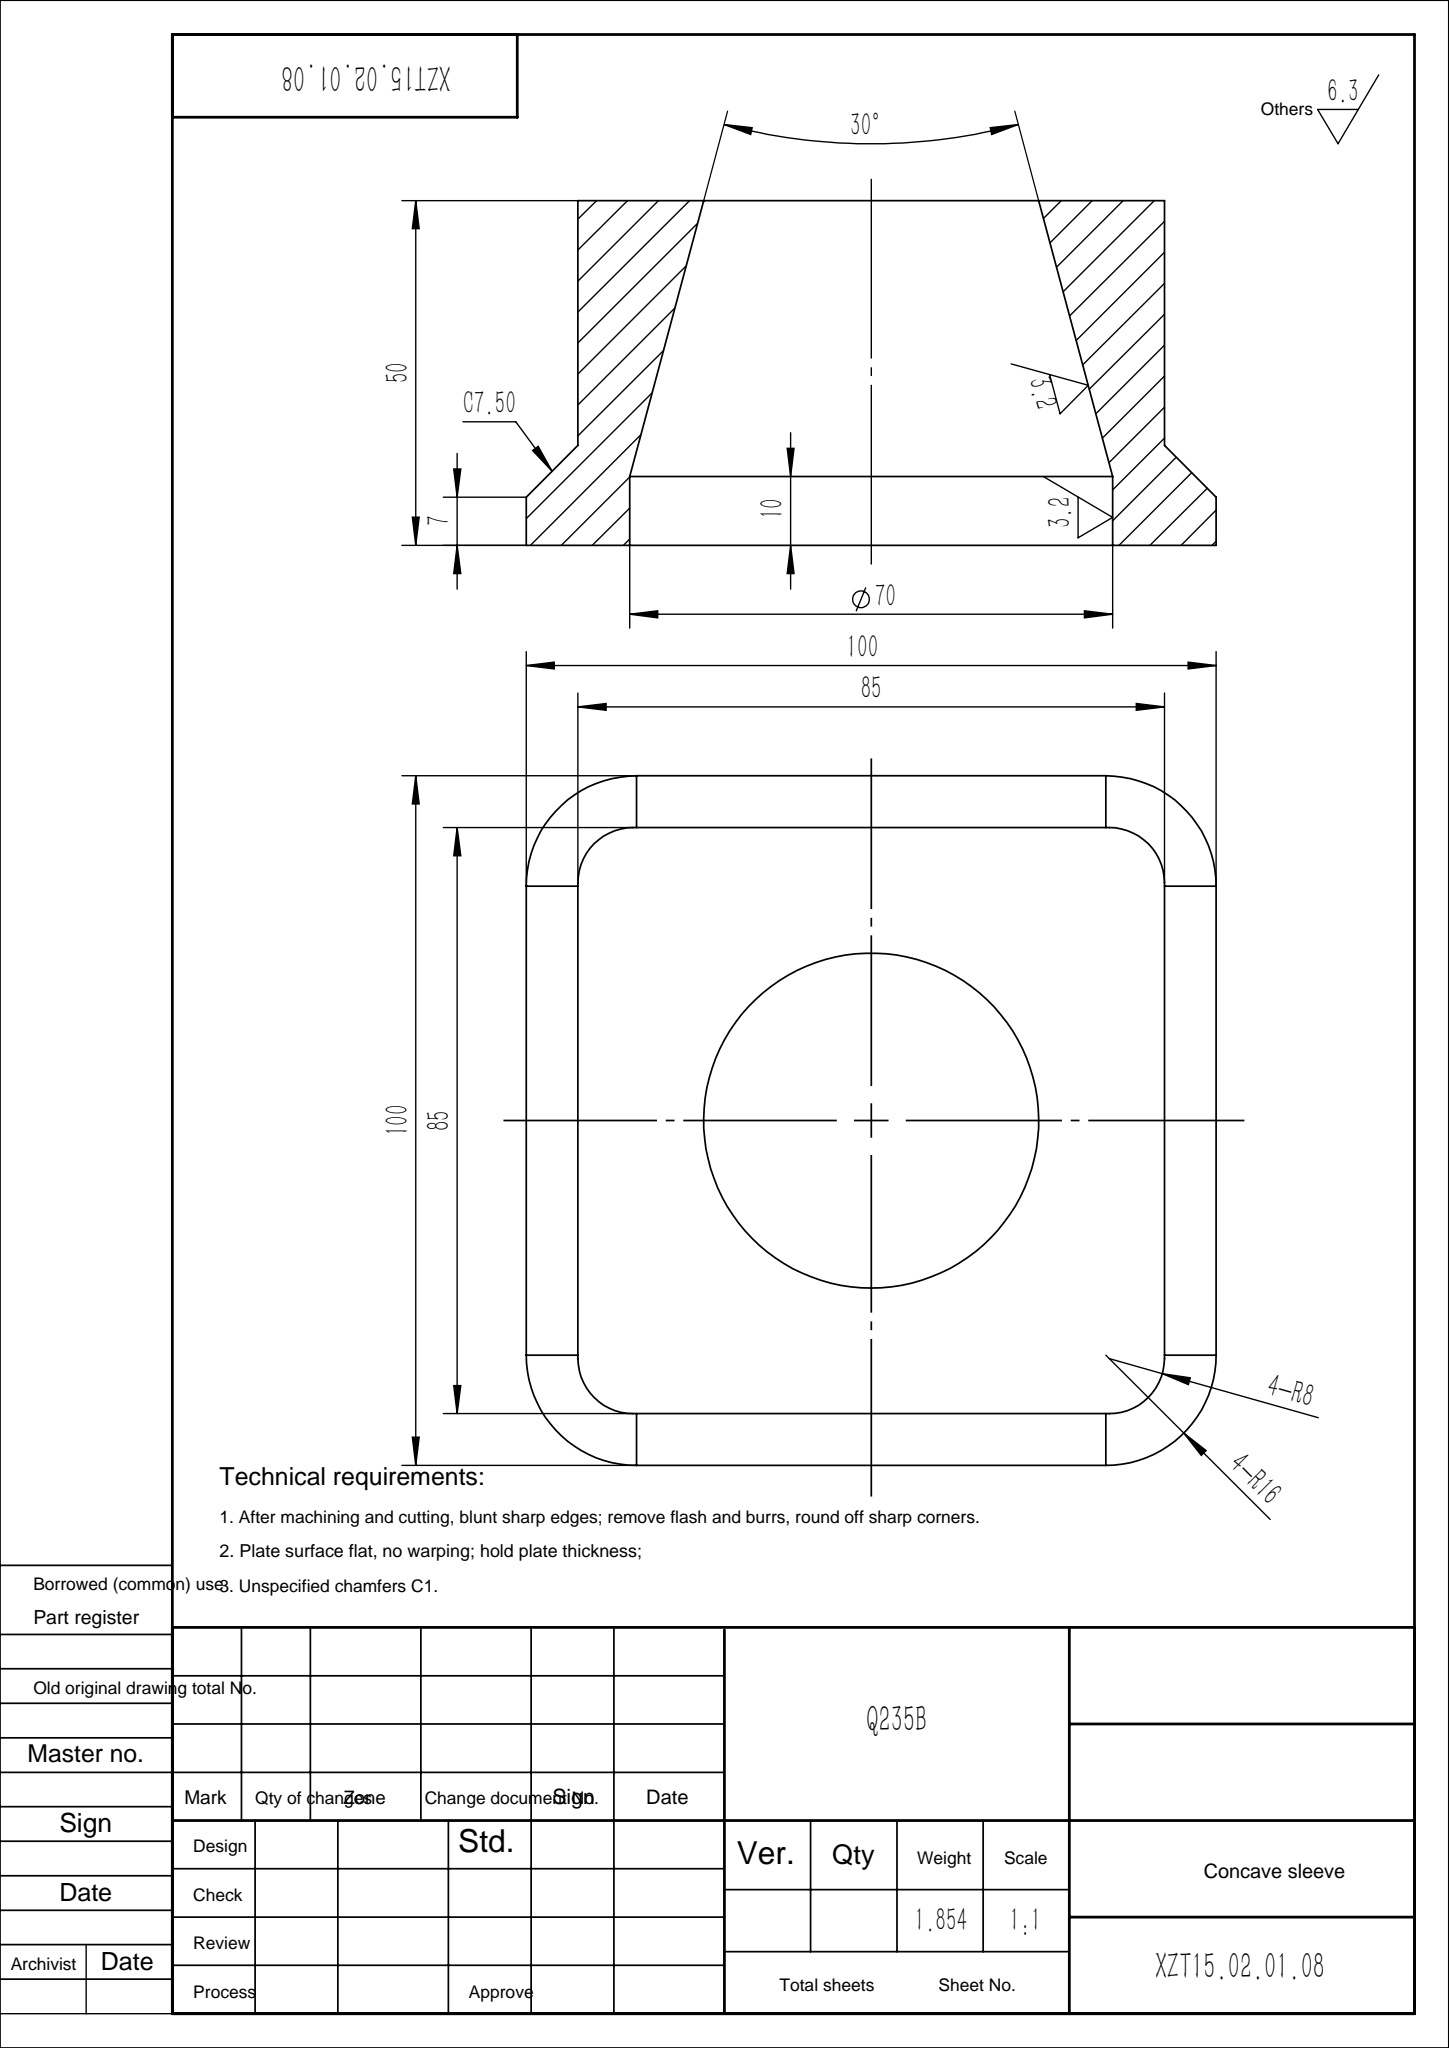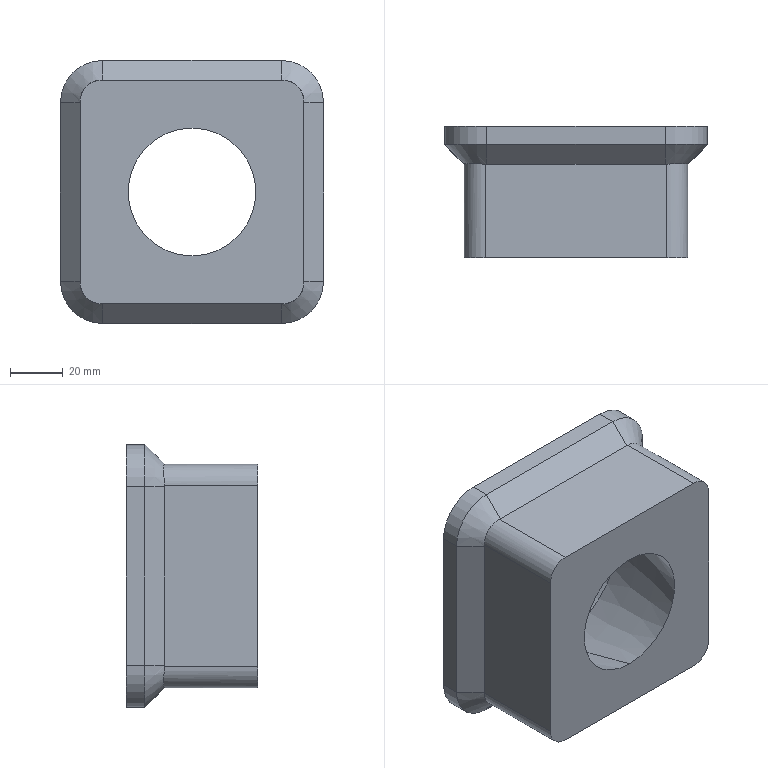Part | SolidWorks | features Chamfer 1, Extrusion 1, ICE 1, RevCut 1 | 1 solid | 30 faces | box 100 x 50 x 100 mm | volume 236221 mm3 | plane 14 | cylinder 10 | cone 6 | commonest cylinder face diameters 16 x4 32 x4 70 x2
STEP:
#1=CARTESIAN_POINT('',(0.,-50.,24.282));
#2=VERTEX_POINT('',#1);
#3=CARTESIAN_POINT('',(0.,-50.,-24.282));
#4=VERTEX_POINT('',#3);
#5=CARTESIAN_POINT('',(0.,-50.,0.));
#6=DIRECTION('',(0.,-1.,0.));
#7=DIRECTION('',(0.,0.,-1.));
#8=AXIS2_PLACEMENT_3D('',#5,#6,#7);
#9=CIRCLE('',#8,24.282);
#10=EDGE_CURVE('',#2,#4,#9,.T.);
#11=ORIENTED_EDGE('',*,*,#10,.T.);
#12=CARTESIAN_POINT('',(0.,-10.,-35.));
#13=VERTEX_POINT('',#12);
#14=CARTESIAN_POINT('',(0.,-10.,-35.));
#15=DIRECTION('',(0.,0.9659,-0.2588));
#16=VECTOR('',#15,1000.);
#17=LINE('',#14,#16);
#18=EDGE_CURVE('',#4,#13,#17,.T.);
#19=ORIENTED_EDGE('',*,*,#18,.T.);
#20=CARTESIAN_POINT('',(0.,-10.,35.));
#21=VERTEX_POINT('',#20);
#22=CARTESIAN_POINT('',(0.,-10.,0.));
#23=DIRECTION('',(0.,-1.,0.));
#24=DIRECTION('',(0.,0.,-1.));
#25=AXIS2_PLACEMENT_3D('',#22,#23,#24);
#26=CIRCLE('',#25,35.);
#27=EDGE_CURVE('',#21,#13,#26,.T.);
#28=ORIENTED_EDGE('',*,*,#27,.F.);
#29=CARTESIAN_POINT('',(0.,-10.,35.));
#30=DIRECTION('',(0.,0.9659,0.2588));
#31=VECTOR('',#30,1000.);
#32=LINE('',#29,#31);
#33=EDGE_CURVE('',#2,#21,#32,.T.);
#34=ORIENTED_EDGE('',*,*,#33,.F.);
#35=EDGE_LOOP('',(#11,#19,#28,#34));
#36=FACE_OUTER_BOUND('',#35,.T.);
#37=CARTESIAN_POINT('',(0.,-10.,0.));
#38=DIRECTION('',(0.,1.,0.));
#39=DIRECTION('',(0.,0.,1.));
#40=AXIS2_PLACEMENT_3D('',#37,#38,#39);
#41=CONICAL_SURFACE('',#40,35.,0.2618);
#42=ADVANCED_FACE('',(#36),#41,.F.);
#43=CARTESIAN_POINT('',(0.,0.,35.));
#44=VERTEX_POINT('',#43);
#45=CARTESIAN_POINT('',(0.,0.,-35.));
#46=VERTEX_POINT('',#45);
#47=CARTESIAN_POINT('',(0.,0.,0.));
#48=DIRECTION('',(0.,-1.,0.));
#49=DIRECTION('',(0.,0.,-1.));
#50=AXIS2_PLACEMENT_3D('',#47,#48,#49);
#51=CIRCLE('',#50,35.);
#52=EDGE_CURVE('',#44,#46,#51,.T.);
#53=ORIENTED_EDGE('',*,*,#52,.F.);
#54=CARTESIAN_POINT('',(0.,-50.,35.));
#55=DIRECTION('',(0.,-1.,0.));
#56=VECTOR('',#55,1000.);
#57=LINE('',#54,#56);
#58=EDGE_CURVE('',#44,#21,#57,.T.);
#59=ORIENTED_EDGE('',*,*,#58,.T.);
#60=ORIENTED_EDGE('',*,*,#27,.T.);
#61=CARTESIAN_POINT('',(0.,-50.,-35.));
#62=DIRECTION('',(0.,-1.,0.));
#63=VECTOR('',#62,1000.);
#64=LINE('',#61,#63);
#65=EDGE_CURVE('',#46,#13,#64,.T.);
#66=ORIENTED_EDGE('',*,*,#65,.F.);
#67=EDGE_LOOP('',(#53,#59,#60,#66));
#68=FACE_OUTER_BOUND('',#67,.T.);
#69=CARTESIAN_POINT('',(0.,-50.,0.));
#70=DIRECTION('',(0.,-1.,0.));
#71=DIRECTION('',(0.,0.,-1.));
#72=AXIS2_PLACEMENT_3D('',#69,#70,#71);
#73=CYLINDRICAL_SURFACE('',#72,35.);
#74=ADVANCED_FACE('',(#68),#73,.F.);
#75=CARTESIAN_POINT('',(-50.,-7.,34.));
#76=VERTEX_POINT('',#75);
#77=CARTESIAN_POINT('',(-50.,0.,34.));
#78=VERTEX_POINT('',#77);
#79=CARTESIAN_POINT('',(-50.,-15.,34.));
#80=DIRECTION('',(0.,1.,0.));
#81=VECTOR('',#80,1000.);
#82=LINE('',#79,#81);
#83=EDGE_CURVE('',#76,#78,#82,.T.);
#84=ORIENTED_EDGE('',*,*,#83,.F.);
#85=CARTESIAN_POINT('',(-34.,-7.,50.));
#86=VERTEX_POINT('',#85);
#87=CARTESIAN_POINT('',(-34.,-7.,34.));
#88=DIRECTION('',(0.,1.,0.));
#89=DIRECTION('',(0.,0.,-1.));
#90=AXIS2_PLACEMENT_3D('',#87,#88,#89);
#91=CIRCLE('',#90,16.);
#92=EDGE_CURVE('',#76,#86,#91,.T.);
#93=ORIENTED_EDGE('',*,*,#92,.T.);
#94=CARTESIAN_POINT('',(-34.,0.,50.));
#95=VERTEX_POINT('',#94);
#96=CARTESIAN_POINT('',(-34.,-15.,50.));
#97=DIRECTION('',(0.,1.,0.));
#98=VECTOR('',#97,1000.);
#99=LINE('',#96,#98);
#100=EDGE_CURVE('',#86,#95,#99,.T.);
#101=ORIENTED_EDGE('',*,*,#100,.T.);
#102=CARTESIAN_POINT('',(-34.,0.,34.));
#103=DIRECTION('',(0.,1.,0.));
#104=DIRECTION('',(0.,0.,-1.));
#105=AXIS2_PLACEMENT_3D('',#102,#103,#104);
#106=CIRCLE('',#105,16.);
#107=EDGE_CURVE('',#78,#95,#106,.T.);
#108=ORIENTED_EDGE('',*,*,#107,.F.);
#109=EDGE_LOOP('',(#84,#93,#101,#108));
#110=FACE_OUTER_BOUND('',#109,.T.);
#111=CARTESIAN_POINT('',(-34.,-15.,34.));
#112=DIRECTION('',(0.,1.,0.));
#113=DIRECTION('',(0.,0.,1.));
#114=AXIS2_PLACEMENT_3D('',#111,#112,#113);
#115=CYLINDRICAL_SURFACE('',#114,16.);
#116=ADVANCED_FACE('',(#110),#115,.T.);
#117=CARTESIAN_POINT('',(-50.,-7.,-34.));
#118=VERTEX_POINT('',#117);
#119=CARTESIAN_POINT('',(-50.,0.,-34.));
#120=VERTEX_POINT('',#119);
#121=CARTESIAN_POINT('',(-50.,-15.,-34.));
#122=DIRECTION('',(0.,1.,0.));
#123=VECTOR('',#122,1000.);
#124=LINE('',#121,#123);
#125=EDGE_CURVE('',#118,#120,#124,.T.);
#126=ORIENTED_EDGE('',*,*,#125,.F.);
#127=CARTESIAN_POINT('',(-50.,-7.,34.));
#128=DIRECTION('',(0.,0.,1.));
#129=VECTOR('',#128,1000.);
#130=LINE('',#127,#129);
#131=EDGE_CURVE('',#118,#76,#130,.T.);
#132=ORIENTED_EDGE('',*,*,#131,.T.);
#133=ORIENTED_EDGE('',*,*,#83,.T.);
#134=CARTESIAN_POINT('',(-50.,0.,34.));
#135=DIRECTION('',(0.,0.,1.));
#136=VECTOR('',#135,1000.);
#137=LINE('',#134,#136);
#138=EDGE_CURVE('',#120,#78,#137,.T.);
#139=ORIENTED_EDGE('',*,*,#138,.F.);
#140=EDGE_LOOP('',(#126,#132,#133,#139));
#141=FACE_OUTER_BOUND('',#140,.T.);
#142=CARTESIAN_POINT('',(-50.,-15.,34.));
#143=DIRECTION('',(-1.,0.,0.));
#144=DIRECTION('',(0.,0.,1.));
#145=AXIS2_PLACEMENT_3D('',#142,#143,#144);
#146=PLANE('',#145);
#147=ADVANCED_FACE('',(#141),#146,.T.);
#148=CARTESIAN_POINT('',(-34.,-7.,-50.));
#149=VERTEX_POINT('',#148);
#150=CARTESIAN_POINT('',(-34.,0.,-50.));
#151=VERTEX_POINT('',#150);
#152=CARTESIAN_POINT('',(-34.,-15.,-50.));
#153=DIRECTION('',(0.,1.,0.));
#154=VECTOR('',#153,1000.);
#155=LINE('',#152,#154);
#156=EDGE_CURVE('',#149,#151,#155,.T.);
#157=ORIENTED_EDGE('',*,*,#156,.F.);
#158=CARTESIAN_POINT('',(-34.,-7.,-34.));
#159=DIRECTION('',(0.,1.,0.));
#160=DIRECTION('',(0.,0.,-1.));
#161=AXIS2_PLACEMENT_3D('',#158,#159,#160);
#162=CIRCLE('',#161,16.);
#163=EDGE_CURVE('',#149,#118,#162,.T.);
#164=ORIENTED_EDGE('',*,*,#163,.T.);
#165=ORIENTED_EDGE('',*,*,#125,.T.);
#166=CARTESIAN_POINT('',(-34.,0.,-34.));
#167=DIRECTION('',(0.,1.,0.));
#168=DIRECTION('',(0.,0.,1.));
#169=AXIS2_PLACEMENT_3D('',#166,#167,#168);
#170=CIRCLE('',#169,16.);
#171=EDGE_CURVE('',#151,#120,#170,.T.);
#172=ORIENTED_EDGE('',*,*,#171,.F.);
#173=EDGE_LOOP('',(#157,#164,#165,#172));
#174=FACE_OUTER_BOUND('',#173,.T.);
#175=CARTESIAN_POINT('',(-34.,-15.,-34.));
#176=DIRECTION('',(0.,1.,0.));
#177=DIRECTION('',(0.,0.,1.));
#178=AXIS2_PLACEMENT_3D('',#175,#176,#177);
#179=CYLINDRICAL_SURFACE('',#178,16.);
#180=ADVANCED_FACE('',(#174),#179,.T.);
#181=CARTESIAN_POINT('',(34.,-7.,-50.));
#182=VERTEX_POINT('',#181);
#183=CARTESIAN_POINT('',(34.,0.,-50.));
#184=VERTEX_POINT('',#183);
#185=CARTESIAN_POINT('',(34.,-15.,-50.));
#186=DIRECTION('',(0.,1.,0.));
#187=VECTOR('',#186,1000.);
#188=LINE('',#185,#187);
#189=EDGE_CURVE('',#182,#184,#188,.T.);
#190=ORIENTED_EDGE('',*,*,#189,.F.);
#191=CARTESIAN_POINT('',(34.,-7.,-50.));
#192=DIRECTION('',(-1.,0.,0.));
#193=VECTOR('',#192,1000.);
#194=LINE('',#191,#193);
#195=EDGE_CURVE('',#182,#149,#194,.T.);
#196=ORIENTED_EDGE('',*,*,#195,.T.);
#197=ORIENTED_EDGE('',*,*,#156,.T.);
#198=CARTESIAN_POINT('',(34.,0.,-50.));
#199=DIRECTION('',(-1.,0.,0.));
#200=VECTOR('',#199,1000.);
#201=LINE('',#198,#200);
#202=EDGE_CURVE('',#184,#151,#201,.T.);
#203=ORIENTED_EDGE('',*,*,#202,.F.);
#204=EDGE_LOOP('',(#190,#196,#197,#203));
#205=FACE_OUTER_BOUND('',#204,.T.);
#206=CARTESIAN_POINT('',(34.,-15.,-50.));
#207=DIRECTION('',(0.,0.,-1.));
#208=DIRECTION('',(-1.,0.,0.));
#209=AXIS2_PLACEMENT_3D('',#206,#207,#208);
#210=PLANE('',#209);
#211=ADVANCED_FACE('',(#205),#210,.T.);
#212=CARTESIAN_POINT('',(50.,-7.,-34.));
#213=VERTEX_POINT('',#212);
#214=CARTESIAN_POINT('',(50.,0.,-34.));
#215=VERTEX_POINT('',#214);
#216=CARTESIAN_POINT('',(50.,-15.,-34.));
#217=DIRECTION('',(0.,1.,0.));
#218=VECTOR('',#217,1000.);
#219=LINE('',#216,#218);
#220=EDGE_CURVE('',#213,#215,#219,.T.);
#221=ORIENTED_EDGE('',*,*,#220,.F.);
#222=CARTESIAN_POINT('',(34.,-7.,-34.));
#223=DIRECTION('',(0.,1.,0.));
#224=DIRECTION('',(0.,0.,-1.));
#225=AXIS2_PLACEMENT_3D('',#222,#223,#224);
#226=CIRCLE('',#225,16.);
#227=EDGE_CURVE('',#213,#182,#226,.T.);
#228=ORIENTED_EDGE('',*,*,#227,.T.);
#229=ORIENTED_EDGE('',*,*,#189,.T.);
#230=CARTESIAN_POINT('',(34.,0.,-34.));
#231=DIRECTION('',(0.,1.,0.));
#232=DIRECTION('',(0.,0.,1.));
#233=AXIS2_PLACEMENT_3D('',#230,#231,#232);
#234=CIRCLE('',#233,16.);
#235=EDGE_CURVE('',#215,#184,#234,.T.);
#236=ORIENTED_EDGE('',*,*,#235,.F.);
#237=EDGE_LOOP('',(#221,#228,#229,#236));
#238=FACE_OUTER_BOUND('',#237,.T.);
#239=CARTESIAN_POINT('',(34.,-15.,-34.));
#240=DIRECTION('',(0.,1.,0.));
#241=DIRECTION('',(0.,0.,1.));
#242=AXIS2_PLACEMENT_3D('',#239,#240,#241);
#243=CYLINDRICAL_SURFACE('',#242,16.);
#244=ADVANCED_FACE('',(#238),#243,.T.);
#245=CARTESIAN_POINT('',(50.,-7.,34.));
#246=VERTEX_POINT('',#245);
#247=CARTESIAN_POINT('',(50.,0.,34.));
#248=VERTEX_POINT('',#247);
#249=CARTESIAN_POINT('',(50.,-15.,34.));
#250=DIRECTION('',(0.,1.,0.));
#251=VECTOR('',#250,1000.);
#252=LINE('',#249,#251);
#253=EDGE_CURVE('',#246,#248,#252,.T.);
#254=ORIENTED_EDGE('',*,*,#253,.F.);
#255=CARTESIAN_POINT('',(50.,-7.,34.));
#256=DIRECTION('',(0.,0.,-1.));
#257=VECTOR('',#256,1000.);
#258=LINE('',#255,#257);
#259=EDGE_CURVE('',#246,#213,#258,.T.);
#260=ORIENTED_EDGE('',*,*,#259,.T.);
#261=ORIENTED_EDGE('',*,*,#220,.T.);
#262=CARTESIAN_POINT('',(50.,0.,34.));
#263=DIRECTION('',(0.,0.,-1.));
#264=VECTOR('',#263,1000.);
#265=LINE('',#262,#264);
#266=EDGE_CURVE('',#248,#215,#265,.T.);
#267=ORIENTED_EDGE('',*,*,#266,.F.);
#268=EDGE_LOOP('',(#254,#260,#261,#267));
#269=FACE_OUTER_BOUND('',#268,.T.);
#270=CARTESIAN_POINT('',(50.,-15.,34.));
#271=DIRECTION('',(1.,0.,0.));
#272=DIRECTION('',(0.,0.,-1.));
#273=AXIS2_PLACEMENT_3D('',#270,#271,#272);
#274=PLANE('',#273);
#275=ADVANCED_FACE('',(#269),#274,.T.);
#276=CARTESIAN_POINT('',(34.,-7.,50.));
#277=VERTEX_POINT('',#276);
#278=CARTESIAN_POINT('',(34.,0.,50.));
#279=VERTEX_POINT('',#278);
#280=CARTESIAN_POINT('',(34.,-15.,50.));
#281=DIRECTION('',(0.,1.,0.));
#282=VECTOR('',#281,1000.);
#283=LINE('',#280,#282);
#284=EDGE_CURVE('',#277,#279,#283,.T.);
#285=ORIENTED_EDGE('',*,*,#284,.F.);
#286=CARTESIAN_POINT('',(34.,-7.,34.));
#287=DIRECTION('',(0.,1.,0.));
#288=DIRECTION('',(0.,0.,-1.));
#289=AXIS2_PLACEMENT_3D('',#286,#287,#288);
#290=CIRCLE('',#289,16.);
#291=EDGE_CURVE('',#277,#246,#290,.T.);
#292=ORIENTED_EDGE('',*,*,#291,.T.);
#293=ORIENTED_EDGE('',*,*,#253,.T.);
#294=CARTESIAN_POINT('',(34.,0.,34.));
#295=DIRECTION('',(0.,1.,0.));
#296=DIRECTION('',(0.,0.,1.));
#297=AXIS2_PLACEMENT_3D('',#294,#295,#296);
#298=CIRCLE('',#297,16.);
#299=EDGE_CURVE('',#279,#248,#298,.T.);
#300=ORIENTED_EDGE('',*,*,#299,.F.);
#301=EDGE_LOOP('',(#285,#292,#293,#300));
#302=FACE_OUTER_BOUND('',#301,.T.);
#303=CARTESIAN_POINT('',(34.,-15.,34.));
#304=DIRECTION('',(0.,1.,0.));
#305=DIRECTION('',(0.,0.,1.));
#306=AXIS2_PLACEMENT_3D('',#303,#304,#305);
#307=CYLINDRICAL_SURFACE('',#306,16.);
#308=ADVANCED_FACE('',(#302),#307,.T.);
#309=ORIENTED_EDGE('',*,*,#100,.F.);
#310=CARTESIAN_POINT('',(34.,-7.,50.));
#311=DIRECTION('',(1.,0.,0.));
#312=VECTOR('',#311,1000.);
#313=LINE('',#310,#312);
#314=EDGE_CURVE('',#86,#277,#313,.T.);
#315=ORIENTED_EDGE('',*,*,#314,.T.);
#316=ORIENTED_EDGE('',*,*,#284,.T.);
#317=CARTESIAN_POINT('',(34.,0.,50.));
#318=DIRECTION('',(1.,0.,0.));
#319=VECTOR('',#318,1000.);
#320=LINE('',#317,#319);
#321=EDGE_CURVE('',#95,#279,#320,.T.);
#322=ORIENTED_EDGE('',*,*,#321,.F.);
#323=EDGE_LOOP('',(#309,#315,#316,#322));
#324=FACE_OUTER_BOUND('',#323,.T.);
#325=CARTESIAN_POINT('',(34.,-15.,50.));
#326=DIRECTION('',(0.,0.,1.));
#327=DIRECTION('',(1.,0.,0.));
#328=AXIS2_PLACEMENT_3D('',#325,#326,#327);
#329=PLANE('',#328);
#330=ADVANCED_FACE('',(#324),#329,.T.);
#331=CARTESIAN_POINT('',(0.,0.,0.));
#332=DIRECTION('',(0.,-1.,0.));
#333=DIRECTION('',(0.,0.,-1.));
#334=AXIS2_PLACEMENT_3D('',#331,#332,#333);
#335=CIRCLE('',#334,35.);
#336=EDGE_CURVE('',#46,#44,#335,.T.);
#337=ORIENTED_EDGE('',*,*,#336,.T.);
#338=ORIENTED_EDGE('',*,*,#52,.T.);
#339=EDGE_LOOP('',(#337,#338));
#340=FACE_BOUND('',#339,.T.);
#341=ORIENTED_EDGE('',*,*,#107,.T.);
#342=ORIENTED_EDGE('',*,*,#321,.T.);
#343=ORIENTED_EDGE('',*,*,#299,.T.);
#344=ORIENTED_EDGE('',*,*,#266,.T.);
#345=ORIENTED_EDGE('',*,*,#235,.T.);
#346=ORIENTED_EDGE('',*,*,#202,.T.);
#347=ORIENTED_EDGE('',*,*,#171,.T.);
#348=ORIENTED_EDGE('',*,*,#138,.T.);
#349=EDGE_LOOP('',(#341,#342,#343,#344,#345,#346,#347,#348));
#350=FACE_OUTER_BOUND('',#349,.T.);
#351=CARTESIAN_POINT('',(-34.,0.,34.));
#352=DIRECTION('',(0.,-1.,0.));
#353=DIRECTION('',(0.,0.,-1.));
#354=AXIS2_PLACEMENT_3D('',#351,#352,#353);
#355=PLANE('',#354);
#356=ADVANCED_FACE('',(#340,#350),#355,.F.);
#357=CARTESIAN_POINT('',(-42.5,-50.,-34.5));
#358=VERTEX_POINT('',#357);
#359=CARTESIAN_POINT('',(-42.5,-14.485,-34.5));
#360=VERTEX_POINT('',#359);
#361=CARTESIAN_POINT('',(-42.5,-50.,-34.5));
#362=DIRECTION('',(0.,1.,0.));
#363=VECTOR('',#362,1000.);
#364=LINE('',#361,#363);
#365=EDGE_CURVE('',#358,#360,#364,.T.);
#366=ORIENTED_EDGE('',*,*,#365,.T.);
#367=CARTESIAN_POINT('',(-34.5,-14.485,-42.5));
#368=VERTEX_POINT('',#367);
#369=CARTESIAN_POINT('',(-42.5,-14.485,-34.5));
#370=CARTESIAN_POINT('',(-42.5,-14.454,-35.028));
#371=CARTESIAN_POINT('',(-42.448,-14.427,-35.547));
#372=CARTESIAN_POINT('',(-42.296,-14.391,-36.314));
#373=CARTESIAN_POINT('',(-42.232,-14.38,-36.568));
#374=CARTESIAN_POINT('',(-42.08,-14.36,-37.072));
#375=CARTESIAN_POINT('',(-41.991,-14.351,-37.321));
#376=CARTESIAN_POINT('',(-41.691,-14.326,-38.045));
#377=CARTESIAN_POINT('',(-41.445,-14.314,-38.505));
#378=CARTESIAN_POINT('',(-41.009,-14.301,-39.158));
#379=CARTESIAN_POINT('',(-40.851,-14.298,-39.371));
#380=CARTESIAN_POINT('',(-40.518,-14.294,-39.778));
#381=CARTESIAN_POINT('',(-40.342,-14.293,-39.971));
#382=CARTESIAN_POINT('',(-39.79,-14.293,-40.524));
#383=CARTESIAN_POINT('',(-39.387,-14.297,-40.856));
#384=CARTESIAN_POINT('',(-38.51,-14.314,-41.443));
#385=CARTESIAN_POINT('',(-38.047,-14.326,-41.689));
#386=CARTESIAN_POINT('',(-37.326,-14.35,-41.989));
#387=CARTESIAN_POINT('',(-37.08,-14.36,-42.077));
#388=CARTESIAN_POINT('',(-36.579,-14.38,-42.23));
#389=CARTESIAN_POINT('',(-36.322,-14.391,-42.294));
#390=CARTESIAN_POINT('',(-35.549,-14.427,-42.448));
#391=CARTESIAN_POINT('',(-35.028,-14.454,-42.5));
#392=CARTESIAN_POINT('',(-34.5,-14.485,-42.5));
#393=B_SPLINE_CURVE_WITH_KNOTS('',3,(#369,#370,#371,#372,#373,#374,#375,#376,#377,#378,#379,#380,#381,#382,#383,#384,#385,#386,#387,#388,#389,#390,#391,#392),.UNSPECIFIED.,.F.,.F.,(4,2,2,2,2,2,2,2,2,2,2,4),(0.,0.001565,0.002348,0.003131,0.004696,0.005479,0.006262,0.007827,0.009393,0.01018,0.01096,0.01252),.UNSPECIFIED.);
#394=EDGE_CURVE('',#360,#368,#393,.T.);
#395=ORIENTED_EDGE('',*,*,#394,.T.);
#396=CARTESIAN_POINT('',(-34.5,-50.,-42.5));
#397=VERTEX_POINT('',#396);
#398=CARTESIAN_POINT('',(-34.5,-50.,-42.5));
#399=DIRECTION('',(0.,1.,0.));
#400=VECTOR('',#399,1000.);
#401=LINE('',#398,#400);
#402=EDGE_CURVE('',#397,#368,#401,.T.);
#403=ORIENTED_EDGE('',*,*,#402,.F.);
#404=CARTESIAN_POINT('',(-34.5,-50.,-34.5));
#405=DIRECTION('',(0.,-1.,0.));
#406=DIRECTION('',(0.,0.,1.));
#407=AXIS2_PLACEMENT_3D('',#404,#405,#406);
#408=CIRCLE('',#407,8.);
#409=EDGE_CURVE('',#358,#397,#408,.T.);
#410=ORIENTED_EDGE('',*,*,#409,.F.);
#411=EDGE_LOOP('',(#366,#395,#403,#410));
#412=FACE_OUTER_BOUND('',#411,.T.);
#413=CARTESIAN_POINT('',(-34.5,-50.,-34.5));
#414=DIRECTION('',(0.,1.,0.));
#415=DIRECTION('',(0.,0.,1.));
#416=AXIS2_PLACEMENT_3D('',#413,#414,#415);
#417=CYLINDRICAL_SURFACE('',#416,8.);
#418=ADVANCED_FACE('',(#412),#417,.T.);
#419=ORIENTED_EDGE('',*,*,#402,.T.);
#420=CARTESIAN_POINT('',(-34.,-14.5,-42.5));
#421=VERTEX_POINT('',#420);
#422=CARTESIAN_POINT('',(-34.5,-14.485,-42.5));
#423=CARTESIAN_POINT('',(-34.333,-14.495,-42.5));
#424=CARTESIAN_POINT('',(-34.166,-14.5,-42.5));
#425=CARTESIAN_POINT('',(-34.,-14.5,-42.5));
#426=B_SPLINE_CURVE_WITH_KNOTS('',3,(#422,#423,#424,#425),.UNSPECIFIED.,.F.,.F.,(4,4),(0.,0.0004968),.UNSPECIFIED.);
#427=EDGE_CURVE('',#368,#421,#426,.T.);
#428=ORIENTED_EDGE('',*,*,#427,.T.);
#429=CARTESIAN_POINT('',(34.,-14.5,-42.5));
#430=VERTEX_POINT('',#429);
#431=CARTESIAN_POINT('',(34.5,-14.5,-42.5));
#432=DIRECTION('',(1.,0.,0.));
#433=VECTOR('',#432,1000.);
#434=LINE('',#431,#433);
#435=EDGE_CURVE('',#421,#430,#434,.T.);
#436=ORIENTED_EDGE('',*,*,#435,.T.);
#437=CARTESIAN_POINT('',(34.5,-14.485,-42.5));
#438=VERTEX_POINT('',#437);
#439=CARTESIAN_POINT('',(34.,-14.5,-42.5));
#440=CARTESIAN_POINT('',(34.167,-14.5,-42.5));
#441=CARTESIAN_POINT('',(34.333,-14.495,-42.5));
#442=CARTESIAN_POINT('',(34.5,-14.485,-42.5));
#443=B_SPLINE_CURVE_WITH_KNOTS('',3,(#439,#440,#441,#442),.UNSPECIFIED.,.F.,.F.,(4,4),(0.,0.0005002),.UNSPECIFIED.);
#444=EDGE_CURVE('',#430,#438,#443,.T.);
#445=ORIENTED_EDGE('',*,*,#444,.T.);
#446=CARTESIAN_POINT('',(34.5,-50.,-42.5));
#447=VERTEX_POINT('',#446);
#448=CARTESIAN_POINT('',(34.5,-50.,-42.5));
#449=DIRECTION('',(0.,1.,0.));
#450=VECTOR('',#449,1000.);
#451=LINE('',#448,#450);
#452=EDGE_CURVE('',#447,#438,#451,.T.);
#453=ORIENTED_EDGE('',*,*,#452,.F.);
#454=CARTESIAN_POINT('',(34.5,-50.,-42.5));
#455=DIRECTION('',(1.,0.,0.));
#456=VECTOR('',#455,1000.);
#457=LINE('',#454,#456);
#458=EDGE_CURVE('',#397,#447,#457,.T.);
#459=ORIENTED_EDGE('',*,*,#458,.F.);
#460=EDGE_LOOP('',(#419,#428,#436,#445,#453,#459));
#461=FACE_OUTER_BOUND('',#460,.T.);
#462=CARTESIAN_POINT('',(34.5,-50.,-42.5));
#463=DIRECTION('',(0.,0.,1.));
#464=DIRECTION('',(1.,0.,0.));
#465=AXIS2_PLACEMENT_3D('',#462,#463,#464);
#466=PLANE('',#465);
#467=ADVANCED_FACE('',(#461),#466,.F.);
#468=ORIENTED_EDGE('',*,*,#452,.T.);
#469=CARTESIAN_POINT('',(42.5,-14.485,-34.5));
#470=VERTEX_POINT('',#469);
#471=CARTESIAN_POINT('',(34.5,-14.485,-42.5));
#472=CARTESIAN_POINT('',(35.027,-14.454,-42.5));
#473=CARTESIAN_POINT('',(35.546,-14.427,-42.448));
#474=CARTESIAN_POINT('',(36.313,-14.391,-42.296));
#475=CARTESIAN_POINT('',(36.567,-14.38,-42.233));
#476=CARTESIAN_POINT('',(37.07,-14.36,-42.08));
#477=CARTESIAN_POINT('',(37.319,-14.351,-41.992));
#478=CARTESIAN_POINT('',(38.043,-14.326,-41.692));
#479=CARTESIAN_POINT('',(38.502,-14.314,-41.447));
#480=CARTESIAN_POINT('',(39.155,-14.301,-41.011));
#481=CARTESIAN_POINT('',(39.368,-14.298,-40.854));
#482=CARTESIAN_POINT('',(39.775,-14.294,-40.52));
#483=CARTESIAN_POINT('',(39.971,-14.293,-40.343));
#484=CARTESIAN_POINT('',(40.531,-14.293,-39.783));
#485=CARTESIAN_POINT('',(40.861,-14.297,-39.379));
#486=CARTESIAN_POINT('',(41.296,-14.309,-38.729));
#487=CARTESIAN_POINT('',(41.43,-14.315,-38.505));
#488=CARTESIAN_POINT('',(41.678,-14.327,-38.041));
#489=CARTESIAN_POINT('',(41.791,-14.334,-37.802));
#490=CARTESIAN_POINT('',(42.091,-14.359,-37.077));
#491=CARTESIAN_POINT('',(42.243,-14.379,-36.58));
#492=CARTESIAN_POINT('',(42.447,-14.427,-35.555));
#493=CARTESIAN_POINT('',(42.5,-14.454,-35.027));
#494=CARTESIAN_POINT('',(42.5,-14.485,-34.5));
#495=B_SPLINE_CURVE_WITH_KNOTS('',3,(#471,#472,#473,#474,#475,#476,#477,#478,#479,#480,#481,#482,#483,#484,#485,#486,#487,#488,#489,#490,#491,#492,#493,#494),.UNSPECIFIED.,.F.,.F.,(4,2,2,2,2,2,2,2,2,2,2,4),(-0.006252,-0.004689,-0.003908,-0.003126,-0.001563,-0.000781,0.000000577,0.001564,0.002345,0.003127,0.00469,0.006254),.UNSPECIFIED.);
#496=EDGE_CURVE('',#438,#470,#495,.T.);
#497=ORIENTED_EDGE('',*,*,#496,.T.);
#498=CARTESIAN_POINT('',(42.5,-50.,-34.5));
#499=VERTEX_POINT('',#498);
#500=CARTESIAN_POINT('',(42.5,-50.,-34.5));
#501=DIRECTION('',(0.,1.,0.));
#502=VECTOR('',#501,1000.);
#503=LINE('',#500,#502);
#504=EDGE_CURVE('',#499,#470,#503,.T.);
#505=ORIENTED_EDGE('',*,*,#504,.F.);
#506=CARTESIAN_POINT('',(34.5,-50.,-34.5));
#507=DIRECTION('',(0.,-1.,0.));
#508=DIRECTION('',(0.,0.,-1.));
#509=AXIS2_PLACEMENT_3D('',#506,#507,#508);
#510=CIRCLE('',#509,8.);
#511=EDGE_CURVE('',#447,#499,#510,.T.);
#512=ORIENTED_EDGE('',*,*,#511,.F.);
#513=EDGE_LOOP('',(#468,#497,#505,#512));
#514=FACE_OUTER_BOUND('',#513,.T.);
#515=CARTESIAN_POINT('',(34.5,-50.,-34.5));
#516=DIRECTION('',(0.,1.,0.));
#517=DIRECTION('',(0.,0.,1.));
#518=AXIS2_PLACEMENT_3D('',#515,#516,#517);
#519=CYLINDRICAL_SURFACE('',#518,8.);
#520=ADVANCED_FACE('',(#514),#519,.T.);
#521=CARTESIAN_POINT('',(42.5,-14.5,-34.));
#522=VERTEX_POINT('',#521);
#523=CARTESIAN_POINT('',(42.5,-14.5,34.));
#524=VERTEX_POINT('',#523);
#525=CARTESIAN_POINT('',(42.5,-14.5,-34.5));
#526=DIRECTION('',(0.,0.,1.));
#527=VECTOR('',#526,1000.);
#528=LINE('',#525,#527);
#529=EDGE_CURVE('',#522,#524,#528,.T.);
#530=ORIENTED_EDGE('',*,*,#529,.T.);
#531=CARTESIAN_POINT('',(42.5,-14.485,34.5));
#532=VERTEX_POINT('',#531);
#533=CARTESIAN_POINT('',(42.5,-14.5,34.));
#534=CARTESIAN_POINT('',(42.5,-14.5,34.167));
#535=CARTESIAN_POINT('',(42.5,-14.495,34.333));
#536=CARTESIAN_POINT('',(42.5,-14.485,34.5));
#537=B_SPLINE_CURVE_WITH_KNOTS('',3,(#533,#534,#535,#536),.UNSPECIFIED.,.F.,.F.,(4,4),(0.,0.0005002),.UNSPECIFIED.);
#538=EDGE_CURVE('',#524,#532,#537,.T.);
#539=ORIENTED_EDGE('',*,*,#538,.T.);
#540=CARTESIAN_POINT('',(42.5,-50.,34.5));
#541=VERTEX_POINT('',#540);
#542=CARTESIAN_POINT('',(42.5,-50.,34.5));
#543=DIRECTION('',(0.,1.,0.));
#544=VECTOR('',#543,1000.);
#545=LINE('',#542,#544);
#546=EDGE_CURVE('',#541,#532,#545,.T.);
#547=ORIENTED_EDGE('',*,*,#546,.F.);
#548=CARTESIAN_POINT('',(42.5,-50.,-34.5));
#549=DIRECTION('',(0.,0.,1.));
#550=VECTOR('',#549,1000.);
#551=LINE('',#548,#550);
#552=EDGE_CURVE('',#499,#541,#551,.T.);
#553=ORIENTED_EDGE('',*,*,#552,.F.);
#554=ORIENTED_EDGE('',*,*,#504,.T.);
#555=CARTESIAN_POINT('',(42.5,-14.485,-34.5));
#556=CARTESIAN_POINT('',(42.5,-14.495,-34.333));
#557=CARTESIAN_POINT('',(42.5,-14.5,-34.166));
#558=CARTESIAN_POINT('',(42.5,-14.5,-34.));
#559=B_SPLINE_CURVE_WITH_KNOTS('',3,(#555,#556,#557,#558),.UNSPECIFIED.,.F.,.F.,(4,4),(0.,0.0004968),.UNSPECIFIED.);
#560=EDGE_CURVE('',#470,#522,#559,.T.);
#561=ORIENTED_EDGE('',*,*,#560,.T.);
#562=EDGE_LOOP('',(#530,#539,#547,#553,#554,#561));
#563=FACE_OUTER_BOUND('',#562,.T.);
#564=CARTESIAN_POINT('',(42.5,-50.,-34.5));
#565=DIRECTION('',(-1.,0.,0.));
#566=DIRECTION('',(0.,0.,1.));
#567=AXIS2_PLACEMENT_3D('',#564,#565,#566);
#568=PLANE('',#567);
#569=ADVANCED_FACE('',(#563),#568,.F.);
#570=ORIENTED_EDGE('',*,*,#546,.T.);
#571=CARTESIAN_POINT('',(34.5,-14.485,42.5));
#572=VERTEX_POINT('',#571);
#573=CARTESIAN_POINT('',(42.5,-14.485,34.5));
#574=CARTESIAN_POINT('',(42.5,-14.454,35.028));
#575=CARTESIAN_POINT('',(42.448,-14.427,35.547));
#576=CARTESIAN_POINT('',(42.296,-14.391,36.314));
#577=CARTESIAN_POINT('',(42.232,-14.38,36.568));
#578=CARTESIAN_POINT('',(42.08,-14.36,37.072));
#579=CARTESIAN_POINT('',(41.991,-14.351,37.321));
#580=CARTESIAN_POINT('',(41.691,-14.326,38.045));
#581=CARTESIAN_POINT('',(41.445,-14.314,38.505));
#582=CARTESIAN_POINT('',(41.009,-14.301,39.158));
#583=CARTESIAN_POINT('',(40.851,-14.298,39.371));
#584=CARTESIAN_POINT('',(40.518,-14.294,39.778));
#585=CARTESIAN_POINT('',(40.342,-14.293,39.971));
#586=CARTESIAN_POINT('',(39.79,-14.293,40.524));
#587=CARTESIAN_POINT('',(39.387,-14.297,40.856));
#588=CARTESIAN_POINT('',(38.51,-14.314,41.443));
#589=CARTESIAN_POINT('',(38.047,-14.326,41.689));
#590=CARTESIAN_POINT('',(37.326,-14.35,41.989));
#591=CARTESIAN_POINT('',(37.08,-14.36,42.077));
#592=CARTESIAN_POINT('',(36.579,-14.38,42.23));
#593=CARTESIAN_POINT('',(36.322,-14.391,42.294));
#594=CARTESIAN_POINT('',(35.549,-14.427,42.448));
#595=CARTESIAN_POINT('',(35.028,-14.454,42.5));
#596=CARTESIAN_POINT('',(34.5,-14.485,42.5));
#597=B_SPLINE_CURVE_WITH_KNOTS('',3,(#573,#574,#575,#576,#577,#578,#579,#580,#581,#582,#583,#584,#585,#586,#587,#588,#589,#590,#591,#592,#593,#594,#595,#596),.UNSPECIFIED.,.F.,.F.,(4,2,2,2,2,2,2,2,2,2,2,4),(0.,0.001565,0.002348,0.003131,0.004696,0.005479,0.006262,0.007827,0.009393,0.01018,0.01096,0.01252),.UNSPECIFIED.);
#598=EDGE_CURVE('',#532,#572,#597,.T.);
#599=ORIENTED_EDGE('',*,*,#598,.T.);
#600=CARTESIAN_POINT('',(34.5,-50.,42.5));
#601=VERTEX_POINT('',#600);
#602=CARTESIAN_POINT('',(34.5,-50.,42.5));
#603=DIRECTION('',(0.,1.,0.));
#604=VECTOR('',#603,1000.);
#605=LINE('',#602,#604);
#606=EDGE_CURVE('',#601,#572,#605,.T.);
#607=ORIENTED_EDGE('',*,*,#606,.F.);
#608=CARTESIAN_POINT('',(34.5,-50.,34.5));
#609=DIRECTION('',(0.,-1.,0.));
#610=DIRECTION('',(0.,0.,-1.));
#611=AXIS2_PLACEMENT_3D('',#608,#609,#610);
#612=CIRCLE('',#611,8.);
#613=EDGE_CURVE('',#541,#601,#612,.T.);
#614=ORIENTED_EDGE('',*,*,#613,.F.);
#615=EDGE_LOOP('',(#570,#599,#607,#614));
#616=FACE_OUTER_BOUND('',#615,.T.);
#617=CARTESIAN_POINT('',(34.5,-50.,34.5));
#618=DIRECTION('',(0.,1.,0.));
#619=DIRECTION('',(0.,0.,1.));
#620=AXIS2_PLACEMENT_3D('',#617,#618,#619);
#621=CYLINDRICAL_SURFACE('',#620,8.);
#622=ADVANCED_FACE('',(#616),#621,.T.);
#623=CARTESIAN_POINT('',(34.,-14.5,42.5));
#624=VERTEX_POINT('',#623);
#625=CARTESIAN_POINT('',(-34.,-14.5,42.5));
#626=VERTEX_POINT('',#625);
#627=CARTESIAN_POINT('',(34.5,-14.5,42.5));
#628=DIRECTION('',(-1.,0.,0.));
#629=VECTOR('',#628,1000.);
#630=LINE('',#627,#629);
#631=EDGE_CURVE('',#624,#626,#630,.T.);
#632=ORIENTED_EDGE('',*,*,#631,.T.);
#633=CARTESIAN_POINT('',(-34.5,-14.485,42.5));
#634=VERTEX_POINT('',#633);
#635=CARTESIAN_POINT('',(-34.,-14.5,42.5));
#636=CARTESIAN_POINT('',(-34.167,-14.5,42.5));
#637=CARTESIAN_POINT('',(-34.333,-14.495,42.5));
#638=CARTESIAN_POINT('',(-34.5,-14.485,42.5));
#639=B_SPLINE_CURVE_WITH_KNOTS('',3,(#635,#636,#637,#638),.UNSPECIFIED.,.F.,.F.,(4,4),(0.,0.0005002),.UNSPECIFIED.);
#640=EDGE_CURVE('',#626,#634,#639,.T.);
#641=ORIENTED_EDGE('',*,*,#640,.T.);
#642=CARTESIAN_POINT('',(-34.5,-50.,42.5));
#643=VERTEX_POINT('',#642);
#644=CARTESIAN_POINT('',(-34.5,-50.,42.5));
#645=DIRECTION('',(0.,1.,0.));
#646=VECTOR('',#645,1000.);
#647=LINE('',#644,#646);
#648=EDGE_CURVE('',#643,#634,#647,.T.);
#649=ORIENTED_EDGE('',*,*,#648,.F.);
#650=CARTESIAN_POINT('',(34.5,-50.,42.5));
#651=DIRECTION('',(-1.,0.,0.));
#652=VECTOR('',#651,1000.);
#653=LINE('',#650,#652);
#654=EDGE_CURVE('',#601,#643,#653,.T.);
#655=ORIENTED_EDGE('',*,*,#654,.F.);
#656=ORIENTED_EDGE('',*,*,#606,.T.);
#657=CARTESIAN_POINT('',(34.5,-14.485,42.5));
#658=CARTESIAN_POINT('',(34.333,-14.495,42.5));
#659=CARTESIAN_POINT('',(34.166,-14.5,42.5));
#660=CARTESIAN_POINT('',(34.,-14.5,42.5));
#661=B_SPLINE_CURVE_WITH_KNOTS('',3,(#657,#658,#659,#660),.UNSPECIFIED.,.F.,.F.,(4,4),(0.,0.0004968),.UNSPECIFIED.);
#662=EDGE_CURVE('',#572,#624,#661,.T.);
#663=ORIENTED_EDGE('',*,*,#662,.T.);
#664=EDGE_LOOP('',(#632,#641,#649,#655,#656,#663));
#665=FACE_OUTER_BOUND('',#664,.T.);
#666=CARTESIAN_POINT('',(34.5,-50.,42.5));
#667=DIRECTION('',(0.,0.,-1.));
#668=DIRECTION('',(-1.,0.,0.));
#669=AXIS2_PLACEMENT_3D('',#666,#667,#668);
#670=PLANE('',#669);
#671=ADVANCED_FACE('',(#665),#670,.F.);
#672=ORIENTED_EDGE('',*,*,#648,.T.);
#673=CARTESIAN_POINT('',(-42.5,-14.485,34.5));
#674=VERTEX_POINT('',#673);
#675=CARTESIAN_POINT('',(-34.5,-14.485,42.5));
#676=CARTESIAN_POINT('',(-35.028,-14.454,42.5));
#677=CARTESIAN_POINT('',(-35.547,-14.427,42.448));
#678=CARTESIAN_POINT('',(-36.314,-14.391,42.296));
#679=CARTESIAN_POINT('',(-36.568,-14.38,42.232));
#680=CARTESIAN_POINT('',(-37.072,-14.36,42.08));
#681=CARTESIAN_POINT('',(-37.321,-14.351,41.991));
#682=CARTESIAN_POINT('',(-38.045,-14.326,41.691));
#683=CARTESIAN_POINT('',(-38.505,-14.314,41.445));
#684=CARTESIAN_POINT('',(-39.158,-14.301,41.009));
#685=CARTESIAN_POINT('',(-39.371,-14.298,40.851));
#686=CARTESIAN_POINT('',(-39.778,-14.294,40.518));
#687=CARTESIAN_POINT('',(-39.971,-14.293,40.342));
#688=CARTESIAN_POINT('',(-40.524,-14.293,39.79));
#689=CARTESIAN_POINT('',(-40.856,-14.297,39.387));
#690=CARTESIAN_POINT('',(-41.443,-14.314,38.51));
#691=CARTESIAN_POINT('',(-41.689,-14.326,38.047));
#692=CARTESIAN_POINT('',(-41.989,-14.35,37.326));
#693=CARTESIAN_POINT('',(-42.077,-14.36,37.08));
#694=CARTESIAN_POINT('',(-42.23,-14.38,36.579));
#695=CARTESIAN_POINT('',(-42.294,-14.391,36.322));
#696=CARTESIAN_POINT('',(-42.448,-14.427,35.549));
#697=CARTESIAN_POINT('',(-42.5,-14.454,35.028));
#698=CARTESIAN_POINT('',(-42.5,-14.485,34.5));
#699=B_SPLINE_CURVE_WITH_KNOTS('',3,(#675,#676,#677,#678,#679,#680,#681,#682,#683,#684,#685,#686,#687,#688,#689,#690,#691,#692,#693,#694,#695,#696,#697,#698),.UNSPECIFIED.,.F.,.F.,(4,2,2,2,2,2,2,2,2,2,2,4),(0.,0.001565,0.002348,0.003131,0.004696,0.005479,0.006262,0.007827,0.009393,0.01018,0.01096,0.01252),.UNSPECIFIED.);
#700=EDGE_CURVE('',#634,#674,#699,.T.);
#701=ORIENTED_EDGE('',*,*,#700,.T.);
#702=CARTESIAN_POINT('',(-42.5,-50.,34.5));
#703=VERTEX_POINT('',#702);
#704=CARTESIAN_POINT('',(-42.5,-50.,34.5));
#705=DIRECTION('',(0.,1.,0.));
#706=VECTOR('',#705,1000.);
#707=LINE('',#704,#706);
#708=EDGE_CURVE('',#703,#674,#707,.T.);
#709=ORIENTED_EDGE('',*,*,#708,.F.);
#710=CARTESIAN_POINT('',(-34.5,-50.,34.5));
#711=DIRECTION('',(0.,-1.,0.));
#712=DIRECTION('',(0.,0.,-1.));
#713=AXIS2_PLACEMENT_3D('',#710,#711,#712);
#714=CIRCLE('',#713,8.);
#715=EDGE_CURVE('',#643,#703,#714,.T.);
#716=ORIENTED_EDGE('',*,*,#715,.F.);
#717=EDGE_LOOP('',(#672,#701,#709,#716));
#718=FACE_OUTER_BOUND('',#717,.T.);
#719=CARTESIAN_POINT('',(-34.5,-50.,34.5));
#720=DIRECTION('',(0.,1.,0.));
#721=DIRECTION('',(0.,0.,1.));
#722=AXIS2_PLACEMENT_3D('',#719,#720,#721);
#723=CYLINDRICAL_SURFACE('',#722,8.);
#724=ADVANCED_FACE('',(#718),#723,.T.);
#725=ORIENTED_EDGE('',*,*,#708,.T.);
#726=CARTESIAN_POINT('',(-42.5,-14.5,34.));
#727=VERTEX_POINT('',#726);
#728=CARTESIAN_POINT('',(-42.5,-14.485,34.5));
#729=CARTESIAN_POINT('',(-42.5,-14.495,34.333));
#730=CARTESIAN_POINT('',(-42.5,-14.5,34.166));
#731=CARTESIAN_POINT('',(-42.5,-14.5,34.));
#732=B_SPLINE_CURVE_WITH_KNOTS('',3,(#728,#729,#730,#731),.UNSPECIFIED.,.F.,.F.,(4,4),(0.,0.0004968),.UNSPECIFIED.);
#733=EDGE_CURVE('',#674,#727,#732,.T.);
#734=ORIENTED_EDGE('',*,*,#733,.T.);
#735=CARTESIAN_POINT('',(-42.5,-14.5,-34.));
#736=VERTEX_POINT('',#735);
#737=CARTESIAN_POINT('',(-42.5,-14.5,-34.5));
#738=DIRECTION('',(0.,0.,-1.));
#739=VECTOR('',#738,1000.);
#740=LINE('',#737,#739);
#741=EDGE_CURVE('',#727,#736,#740,.T.);
#742=ORIENTED_EDGE('',*,*,#741,.T.);
#743=CARTESIAN_POINT('',(-42.5,-14.5,-34.));
#744=CARTESIAN_POINT('',(-42.5,-14.5,-34.167));
#745=CARTESIAN_POINT('',(-42.5,-14.495,-34.333));
#746=CARTESIAN_POINT('',(-42.5,-14.485,-34.5));
#747=B_SPLINE_CURVE_WITH_KNOTS('',3,(#743,#744,#745,#746),.UNSPECIFIED.,.F.,.F.,(4,4),(0.,0.0005002),.UNSPECIFIED.);
#748=EDGE_CURVE('',#736,#360,#747,.T.);
#749=ORIENTED_EDGE('',*,*,#748,.T.);
#750=ORIENTED_EDGE('',*,*,#365,.F.);
#751=CARTESIAN_POINT('',(-42.5,-50.,-34.5));
#752=DIRECTION('',(0.,0.,-1.));
#753=VECTOR('',#752,1000.);
#754=LINE('',#751,#753);
#755=EDGE_CURVE('',#703,#358,#754,.T.);
#756=ORIENTED_EDGE('',*,*,#755,.F.);
#757=EDGE_LOOP('',(#725,#734,#742,#749,#750,#756));
#758=FACE_OUTER_BOUND('',#757,.T.);
#759=CARTESIAN_POINT('',(-42.5,-50.,-34.5));
#760=DIRECTION('',(1.,0.,0.));
#761=DIRECTION('',(0.,0.,-1.));
#762=AXIS2_PLACEMENT_3D('',#759,#760,#761);
#763=PLANE('',#762);
#764=ADVANCED_FACE('',(#758),#763,.F.);
#765=ORIENTED_EDGE('',*,*,#10,.F.);
#766=CARTESIAN_POINT('',(0.,-50.,0.));
#767=DIRECTION('',(0.,-1.,0.));
#768=DIRECTION('',(0.,0.,-1.));
#769=AXIS2_PLACEMENT_3D('',#766,#767,#768);
#770=CIRCLE('',#769,24.282);
#771=EDGE_CURVE('',#4,#2,#770,.T.);
#772=ORIENTED_EDGE('',*,*,#771,.F.);
#773=EDGE_LOOP('',(#765,#772));
#774=FACE_BOUND('',#773,.T.);
#775=ORIENTED_EDGE('',*,*,#409,.T.);
#776=ORIENTED_EDGE('',*,*,#458,.T.);
#777=ORIENTED_EDGE('',*,*,#511,.T.);
#778=ORIENTED_EDGE('',*,*,#552,.T.);
#779=ORIENTED_EDGE('',*,*,#613,.T.);
#780=ORIENTED_EDGE('',*,*,#654,.T.);
#781=ORIENTED_EDGE('',*,*,#715,.T.);
#782=ORIENTED_EDGE('',*,*,#755,.T.);
#783=EDGE_LOOP('',(#775,#776,#777,#778,#779,#780,#781,#782));
#784=FACE_OUTER_BOUND('',#783,.T.);
#785=CARTESIAN_POINT('',(-34.5,-50.,-34.5));
#786=DIRECTION('',(0.,1.,0.));
#787=DIRECTION('',(0.,0.,1.));
#788=AXIS2_PLACEMENT_3D('',#785,#786,#787);
#789=PLANE('',#788);
#790=ADVANCED_FACE('',(#774,#784),#789,.F.);
#791=ORIENTED_EDGE('',*,*,#58,.F.);
#792=ORIENTED_EDGE('',*,*,#336,.F.);
#793=ORIENTED_EDGE('',*,*,#65,.T.);
#794=CARTESIAN_POINT('',(0.,-10.,0.));
#795=DIRECTION('',(0.,-1.,0.));
#796=DIRECTION('',(0.,0.,-1.));
#797=AXIS2_PLACEMENT_3D('',#794,#795,#796);
#798=CIRCLE('',#797,35.);
#799=EDGE_CURVE('',#13,#21,#798,.T.);
#800=ORIENTED_EDGE('',*,*,#799,.T.);
#801=EDGE_LOOP('',(#791,#792,#793,#800));
#802=FACE_OUTER_BOUND('',#801,.T.);
#803=CARTESIAN_POINT('',(0.,-50.,0.));
#804=DIRECTION('',(0.,-1.,0.));
#805=DIRECTION('',(0.,0.,-1.));
#806=AXIS2_PLACEMENT_3D('',#803,#804,#805);
#807=CYLINDRICAL_SURFACE('',#806,35.);
#808=ADVANCED_FACE('',(#802),#807,.F.);
#809=ORIENTED_EDGE('',*,*,#18,.F.);
#810=ORIENTED_EDGE('',*,*,#771,.T.);
#811=ORIENTED_EDGE('',*,*,#33,.T.);
#812=ORIENTED_EDGE('',*,*,#799,.F.);
#813=EDGE_LOOP('',(#809,#810,#811,#812));
#814=FACE_OUTER_BOUND('',#813,.T.);
#815=CARTESIAN_POINT('',(0.,-10.,0.));
#816=DIRECTION('',(0.,1.,0.));
#817=DIRECTION('',(0.,0.,1.));
#818=AXIS2_PLACEMENT_3D('',#815,#816,#817);
#819=CONICAL_SURFACE('',#818,35.,0.2618);
#820=ADVANCED_FACE('',(#814),#819,.F.);
#821=ORIENTED_EDGE('',*,*,#700,.F.);
#822=ORIENTED_EDGE('',*,*,#640,.F.);
#823=CARTESIAN_POINT('',(-34.,-7.,50.));
#824=DIRECTION('',(0.,-0.7071,-0.7071));
#825=VECTOR('',#824,1000.);
#826=LINE('',#823,#825);
#827=EDGE_CURVE('',#86,#626,#826,.T.);
#828=ORIENTED_EDGE('',*,*,#827,.F.);
#829=ORIENTED_EDGE('',*,*,#92,.F.);
#830=CARTESIAN_POINT('',(-42.,-15.,34.));
#831=DIRECTION('',(-0.7071,0.7071,0.));
#832=VECTOR('',#831,1000.);
#833=LINE('',#830,#832);
#834=EDGE_CURVE('',#727,#76,#833,.T.);
#835=ORIENTED_EDGE('',*,*,#834,.F.);
#836=ORIENTED_EDGE('',*,*,#733,.F.);
#837=EDGE_LOOP('',(#821,#822,#828,#829,#835,#836));
#838=FACE_OUTER_BOUND('',#837,.T.);
#839=CARTESIAN_POINT('',(-34.,-7.,34.));
#840=DIRECTION('',(0.,1.,0.));
#841=DIRECTION('',(0.,0.,1.));
#842=AXIS2_PLACEMENT_3D('',#839,#840,#841);
#843=CONICAL_SURFACE('',#842,16.,0.7854);
#844=ADVANCED_FACE('',(#838),#843,.T.);
#845=ORIENTED_EDGE('',*,*,#827,.T.);
#846=ORIENTED_EDGE('',*,*,#631,.F.);
#847=CARTESIAN_POINT('',(34.,-7.,50.));
#848=DIRECTION('',(0.,-0.7071,-0.7071));
#849=VECTOR('',#848,1000.);
#850=LINE('',#847,#849);
#851=EDGE_CURVE('',#277,#624,#850,.T.);
#852=ORIENTED_EDGE('',*,*,#851,.F.);
#853=ORIENTED_EDGE('',*,*,#314,.F.);
#854=EDGE_LOOP('',(#845,#846,#852,#853));
#855=FACE_OUTER_BOUND('',#854,.T.);
#856=CARTESIAN_POINT('',(34.,-7.,50.));
#857=DIRECTION('',(0.,0.7071,-0.7071));
#858=DIRECTION('',(1.,0.,0.));
#859=AXIS2_PLACEMENT_3D('',#856,#857,#858);
#860=PLANE('',#859);
#861=ADVANCED_FACE('',(#855),#860,.F.);
#862=ORIENTED_EDGE('',*,*,#834,.T.);
#863=ORIENTED_EDGE('',*,*,#131,.F.);
#864=CARTESIAN_POINT('',(-42.,-15.,-34.));
#865=DIRECTION('',(-0.7071,0.7071,0.));
#866=VECTOR('',#865,1000.);
#867=LINE('',#864,#866);
#868=EDGE_CURVE('',#736,#118,#867,.T.);
#869=ORIENTED_EDGE('',*,*,#868,.F.);
#870=ORIENTED_EDGE('',*,*,#741,.F.);
#871=EDGE_LOOP('',(#862,#863,#869,#870));
#872=FACE_OUTER_BOUND('',#871,.T.);
#873=CARTESIAN_POINT('',(-50.,-7.,34.));
#874=DIRECTION('',(0.7071,0.7071,0.));
#875=DIRECTION('',(0.,0.,1.));
#876=AXIS2_PLACEMENT_3D('',#873,#874,#875);
#877=PLANE('',#876);
#878=ADVANCED_FACE('',(#872),#877,.F.);
#879=ORIENTED_EDGE('',*,*,#598,.F.);
#880=ORIENTED_EDGE('',*,*,#538,.F.);
#881=CARTESIAN_POINT('',(50.,-7.,34.));
#882=DIRECTION('',(-0.7071,-0.7071,0.));
#883=VECTOR('',#882,1000.);
#884=LINE('',#881,#883);
#885=EDGE_CURVE('',#246,#524,#884,.T.);
#886=ORIENTED_EDGE('',*,*,#885,.F.);
#887=ORIENTED_EDGE('',*,*,#291,.F.);
#888=ORIENTED_EDGE('',*,*,#851,.T.);
#889=ORIENTED_EDGE('',*,*,#662,.F.);
#890=EDGE_LOOP('',(#879,#880,#886,#887,#888,#889));
#891=FACE_OUTER_BOUND('',#890,.T.);
#892=CARTESIAN_POINT('',(34.,-7.,34.));
#893=DIRECTION('',(0.,1.,0.));
#894=DIRECTION('',(0.,0.,1.));
#895=AXIS2_PLACEMENT_3D('',#892,#893,#894);
#896=CONICAL_SURFACE('',#895,16.,0.7854);
#897=ADVANCED_FACE('',(#891),#896,.T.);
#898=ORIENTED_EDGE('',*,*,#868,.T.);
#899=ORIENTED_EDGE('',*,*,#163,.F.);
#900=CARTESIAN_POINT('',(-34.,-15.,-42.));
#901=DIRECTION('',(0.,0.7071,-0.7071));
#902=VECTOR('',#901,1000.);
#903=LINE('',#900,#902);
#904=EDGE_CURVE('',#421,#149,#903,.T.);
#905=ORIENTED_EDGE('',*,*,#904,.F.);
#906=ORIENTED_EDGE('',*,*,#427,.F.);
#907=ORIENTED_EDGE('',*,*,#394,.F.);
#908=ORIENTED_EDGE('',*,*,#748,.F.);
#909=EDGE_LOOP('',(#898,#899,#905,#906,#907,#908));
#910=FACE_OUTER_BOUND('',#909,.T.);
#911=CARTESIAN_POINT('',(-34.,-7.,-34.));
#912=DIRECTION('',(0.,1.,0.));
#913=DIRECTION('',(0.,0.,1.));
#914=AXIS2_PLACEMENT_3D('',#911,#912,#913);
#915=CONICAL_SURFACE('',#914,16.,0.7854);
#916=ADVANCED_FACE('',(#910),#915,.T.);
#917=ORIENTED_EDGE('',*,*,#885,.T.);
#918=ORIENTED_EDGE('',*,*,#529,.F.);
#919=CARTESIAN_POINT('',(50.,-7.,-34.));
#920=DIRECTION('',(-0.7071,-0.7071,0.));
#921=VECTOR('',#920,1000.);
#922=LINE('',#919,#921);
#923=EDGE_CURVE('',#213,#522,#922,.T.);
#924=ORIENTED_EDGE('',*,*,#923,.F.);
#925=ORIENTED_EDGE('',*,*,#259,.F.);
#926=EDGE_LOOP('',(#917,#918,#924,#925));
#927=FACE_OUTER_BOUND('',#926,.T.);
#928=CARTESIAN_POINT('',(50.,-7.,34.));
#929=DIRECTION('',(-0.7071,0.7071,0.));
#930=DIRECTION('',(0.,0.,-1.));
#931=AXIS2_PLACEMENT_3D('',#928,#929,#930);
#932=PLANE('',#931);
#933=ADVANCED_FACE('',(#927),#932,.F.);
#934=ORIENTED_EDGE('',*,*,#904,.T.);
#935=ORIENTED_EDGE('',*,*,#195,.F.);
#936=CARTESIAN_POINT('',(34.,-15.,-42.));
#937=DIRECTION('',(0.,0.7071,-0.7071));
#938=VECTOR('',#937,1000.);
#939=LINE('',#936,#938);
#940=EDGE_CURVE('',#430,#182,#939,.T.);
#941=ORIENTED_EDGE('',*,*,#940,.F.);
#942=ORIENTED_EDGE('',*,*,#435,.F.);
#943=EDGE_LOOP('',(#934,#935,#941,#942));
#944=FACE_OUTER_BOUND('',#943,.T.);
#945=CARTESIAN_POINT('',(34.,-7.,-50.));
#946=DIRECTION('',(0.,0.7071,0.7071));
#947=DIRECTION('',(-1.,0.,0.));
#948=AXIS2_PLACEMENT_3D('',#945,#946,#947);
#949=PLANE('',#948);
#950=ADVANCED_FACE('',(#944),#949,.F.);
#951=ORIENTED_EDGE('',*,*,#227,.F.);
#952=ORIENTED_EDGE('',*,*,#923,.T.);
#953=ORIENTED_EDGE('',*,*,#560,.F.);
#954=ORIENTED_EDGE('',*,*,#496,.F.);
#955=ORIENTED_EDGE('',*,*,#444,.F.);
#956=ORIENTED_EDGE('',*,*,#940,.T.);
#957=EDGE_LOOP('',(#951,#952,#953,#954,#955,#956));
#958=FACE_OUTER_BOUND('',#957,.T.);
#959=CARTESIAN_POINT('',(34.,-7.,-34.));
#960=DIRECTION('',(0.,1.,0.));
#961=DIRECTION('',(0.,0.,1.));
#962=AXIS2_PLACEMENT_3D('',#959,#960,#961);
#963=CONICAL_SURFACE('',#962,16.,0.7854);
#964=ADVANCED_FACE('',(#958),#963,.T.);
#965=CLOSED_SHELL('',(#42,#74,#116,#147,#180,#211,#244,#275,#308,#330,#356,#418,#467,#520,#569,#622,#671,#724,#764,#790,#808,#820,#844,#861,#878,#897,#916,#933,#950,#964));
#966=MANIFOLD_SOLID_BREP('',#965);
#967=CARTESIAN_POINT('',(0.,0.,0.));
#968=DIRECTION('',(0.,0.,1.));
#969=DIRECTION('',(1.,0.,0.));
#970=AXIS2_PLACEMENT_3D('',#967,#968,#969);
#971=(LENGTH_UNIT()NAMED_UNIT(*)SI_UNIT(.MILLI.,.METRE.));
#972=UNCERTAINTY_MEASURE_WITH_UNIT(LENGTH_MEASURE(0.00001),#971,'','');
#973=(NAMED_UNIT(*)PLANE_ANGLE_UNIT()SI_UNIT($,.RADIAN.));
#974=(NAMED_UNIT(*)SI_UNIT($,.STERADIAN.)SOLID_ANGLE_UNIT());
#975=(GEOMETRIC_REPRESENTATION_CONTEXT(3)GLOBAL_UNCERTAINTY_ASSIGNED_CONTEXT((#972))GLOBAL_UNIT_ASSIGNED_CONTEXT((#971,#973,#974))REPRESENTATION_CONTEXT('',''));
#976=ADVANCED_BREP_SHAPE_REPRESENTATION('',(#966,#970),#975);